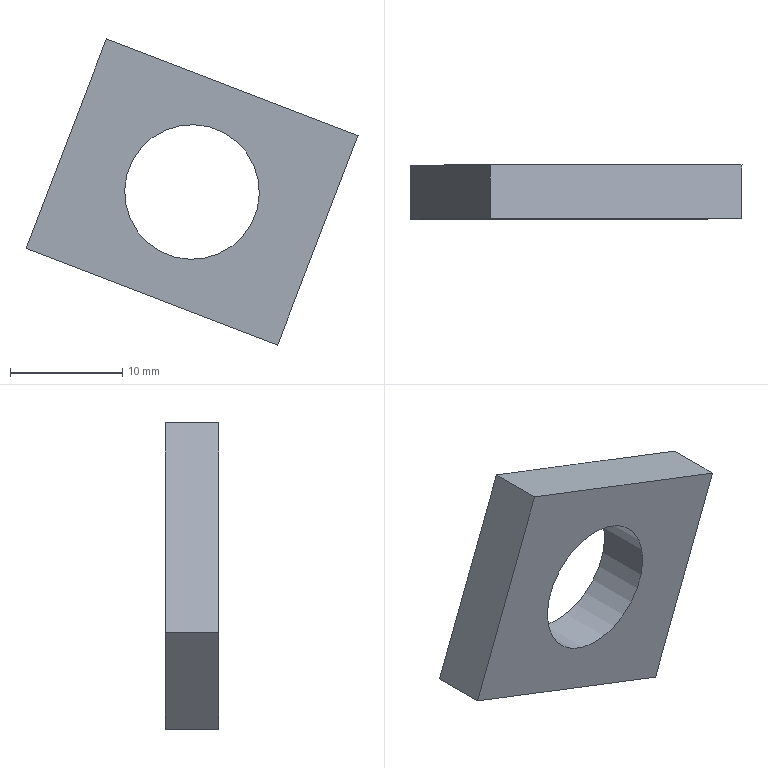Part | STEP file | P011002L001-005 | 1 solid | 7 faces | box 29.573 x 4.8 x 27.272 mm | volume 1761 mm3 | plane 6 | cylinder 1 | commonest cylinder face diameters 12 x1
STEP:
#1=CARTESIAN_POINT('',(0.,0.,0.));
#2=DIRECTION('',(0.,0.,1.));
#3=DIRECTION('',(1.,0.,0.));
#4=AXIS2_PLACEMENT_3D('',#1,#2,#3);
#5=CARTESIAN_POINT('',(-86.963,86.76,-310.6));
#6=VERTEX_POINT('',#5);
#7=CARTESIAN_POINT('',(-64.557,86.76,-319.201));
#8=VERTEX_POINT('',#7);
#9=CARTESIAN_POINT('',(-86.963,86.76,-310.6));
#10=DIRECTION('',(0.9336,0.000000025,-0.3584));
#11=VECTOR('',#10,1.);
#12=LINE('',#9,#11);
#13=CARTESIAN_POINT('',(-77.518,86.76,-285.304));
#14=DIRECTION('',(0.00000001,1.,0.000000094));
#15=DIRECTION('',(0.2588,-0.000000093,0.9659));
#16=AXIS2_PLACEMENT_3D('',#13,#14,#15);
#17=PLANE('',#16);
#18=CARTESIAN_POINT('',(-26.878,-2.576));
#19=DIRECTION('',(-0.1045,0.9945));
#20=VECTOR('',#19,1.);
#21=LINE('',#18,#20);
#22=(GEOMETRIC_REPRESENTATION_CONTEXT(2)PARAMETRIC_REPRESENTATION_CONTEXT()REPRESENTATION_CONTEXT('',''));
#23=DEFINITIONAL_REPRESENTATION('',(#21),#22);
#24=PCURVE('',#17,#23);
#25=CARTESIAN_POINT('',(-86.963,112.76,-310.6));
#26=DIRECTION('',(-0.3584,0.000000186,-0.9336));
#27=DIRECTION('',(-0.9336,-0.000000025,0.3584));
#28=AXIS2_PLACEMENT_3D('',#25,#26,#27);
#29=PLANE('',#28);
#30=CARTESIAN_POINT('',(0.,-26.));
#31=DIRECTION('',(-1.,0.));
#32=VECTOR('',#31,1.);
#33=LINE('',#30,#32);
#34=(GEOMETRIC_REPRESENTATION_CONTEXT(2)PARAMETRIC_REPRESENTATION_CONTEXT()REPRESENTATION_CONTEXT('',''));
#35=DEFINITIONAL_REPRESENTATION('',(#33),#34);
#36=PCURVE('',#29,#35);
#37=SURFACE_CURVE('',#12,(#24,#36),.PCURVE_S1.);
#38=EDGE_CURVE('',#6,#8,#37,.T.);
#39=ORIENTED_EDGE('',*,*,#38,.F.);
#40=CARTESIAN_POINT('',(-79.795,86.76,-291.928));
#41=VERTEX_POINT('',#40);
#42=CARTESIAN_POINT('',(-79.795,86.76,-291.928));
#43=DIRECTION('',(-0.3584,0.000000091,-0.9336));
#44=VECTOR('',#43,1.);
#45=LINE('',#42,#44);
#46=CARTESIAN_POINT('',(-6.988,-0.4856));
#47=DIRECTION('',(-0.9945,-0.1045));
#48=VECTOR('',#47,1.);
#49=LINE('',#46,#48);
#50=(GEOMETRIC_REPRESENTATION_CONTEXT(2)PARAMETRIC_REPRESENTATION_CONTEXT()REPRESENTATION_CONTEXT('',''));
#51=DEFINITIONAL_REPRESENTATION('',(#49),#50);
#52=PCURVE('',#17,#51);
#53=CARTESIAN_POINT('',(-79.795,112.76,-291.928));
#54=DIRECTION('',(-0.9336,-0.000000025,0.3584));
#55=DIRECTION('',(0.3584,-0.000000186,0.9336));
#56=AXIS2_PLACEMENT_3D('',#53,#54,#55);
#57=PLANE('',#56);
#58=CARTESIAN_POINT('',(0.000002462,-26.));
#59=DIRECTION('',(-1.,-0.000000095));
#60=VECTOR('',#59,1.);
#61=LINE('',#58,#60);
#62=(GEOMETRIC_REPRESENTATION_CONTEXT(2)PARAMETRIC_REPRESENTATION_CONTEXT()REPRESENTATION_CONTEXT('',''));
#63=DEFINITIONAL_REPRESENTATION('',(#61),#62);
#64=PCURVE('',#57,#63);
#65=SURFACE_CURVE('',#45,(#52,#64),.PCURVE_S1.);
#66=EDGE_CURVE('',#41,#6,#65,.T.);
#67=ORIENTED_EDGE('',*,*,#66,.F.);
#68=CARTESIAN_POINT('',(-57.389,86.76,-300.529));
#69=VERTEX_POINT('',#68);
#70=CARTESIAN_POINT('',(-80.026,86.76,-291.839));
#71=DIRECTION('',(0.9336,0.000000025,-0.3584));
#72=VECTOR('',#71,1.);
#73=LINE('',#70,#72);
#74=CARTESIAN_POINT('',(-6.962,-0.7317));
#75=DIRECTION('',(-0.1045,0.9945));
#76=VECTOR('',#75,1.);
#77=LINE('',#74,#76);
#78=(GEOMETRIC_REPRESENTATION_CONTEXT(2)PARAMETRIC_REPRESENTATION_CONTEXT()REPRESENTATION_CONTEXT('',''));
#79=DEFINITIONAL_REPRESENTATION('',(#77),#78);
#80=PCURVE('',#17,#79);
#81=CARTESIAN_POINT('',(-57.389,112.76,-300.529));
#82=DIRECTION('',(0.3584,-0.000000186,0.9336));
#83=DIRECTION('',(0.9336,0.000000025,-0.3584));
#84=AXIS2_PLACEMENT_3D('',#81,#82,#83);
#85=PLANE('',#84);
#86=CARTESIAN_POINT('',(-24.247,-26.));
#87=DIRECTION('',(1.,0.));
#88=VECTOR('',#87,1.);
#89=LINE('',#86,#88);
#90=(GEOMETRIC_REPRESENTATION_CONTEXT(2)PARAMETRIC_REPRESENTATION_CONTEXT()REPRESENTATION_CONTEXT('',''));
#91=DEFINITIONAL_REPRESENTATION('',(#89),#90);
#92=PCURVE('',#85,#91);
#93=SURFACE_CURVE('',#73,(#80,#92),.PCURVE_S1.);
#94=EDGE_CURVE('',#41,#69,#93,.T.);
#95=ORIENTED_EDGE('',*,*,#94,.T.);
#96=CARTESIAN_POINT('',(-54.881,86.76,-293.994));
#97=DIRECTION('',(-0.3584,0.000000091,-0.9336));
#98=VECTOR('',#97,1.);
#99=LINE('',#96,#98);
#100=CARTESIAN_POINT('',(-2.535,24.115));
#101=DIRECTION('',(-0.9945,-0.1045));
#102=VECTOR('',#101,1.);
#103=LINE('',#100,#102);
#104=(GEOMETRIC_REPRESENTATION_CONTEXT(2)PARAMETRIC_REPRESENTATION_CONTEXT()REPRESENTATION_CONTEXT('',''));
#105=DEFINITIONAL_REPRESENTATION('',(#103),#104);
#106=PCURVE('',#17,#105);
#107=CARTESIAN_POINT('',(-64.557,112.76,-319.201));
#108=DIRECTION('',(0.9336,0.000000025,-0.3584));
#109=DIRECTION('',(-0.3584,0.000000186,-0.9336));
#110=AXIS2_PLACEMENT_3D('',#107,#108,#109);
#111=PLANE('',#110);
#112=CARTESIAN_POINT('',(-27.,-26.));
#113=DIRECTION('',(1.,-0.000000095));
#114=VECTOR('',#113,1.);
#115=LINE('',#112,#114);
#116=(GEOMETRIC_REPRESENTATION_CONTEXT(2)PARAMETRIC_REPRESENTATION_CONTEXT()REPRESENTATION_CONTEXT('',''));
#117=DEFINITIONAL_REPRESENTATION('',(#115),#116);
#118=PCURVE('',#111,#117);
#119=SURFACE_CURVE('',#99,(#106,#118),.PCURVE_S1.);
#120=EDGE_CURVE('',#69,#8,#119,.T.);
#121=ORIENTED_EDGE('',*,*,#120,.T.);
#122=EDGE_LOOP('',(#39,#67,#95,#121));
#123=FACE_BOUND('',#122,.T.);
#124=CARTESIAN_POINT('',(-70.623,86.76,-299.769));
#125=VERTEX_POINT('',#124);
#126=CARTESIAN_POINT('',(-72.176,86.76,-305.564));
#127=DIRECTION('',(-0.00000001,-1.,-0.000000094));
#128=DIRECTION('',(0.2588,-0.000000093,0.9659));
#129=AXIS2_PLACEMENT_3D('',#126,#127,#128);
#130=CIRCLE('',#129,6.);
#131=CARTESIAN_POINT('',(-12.187,10.403));
#132=CARTESIAN_POINT('',(-12.187,0.01107));
#133=CARTESIAN_POINT('',(-21.187,5.207));
#134=CARTESIAN_POINT('',(-30.187,10.403));
#135=CARTESIAN_POINT('',(-21.187,15.6));
#136=CARTESIAN_POINT('',(-12.187,20.796));
#137=CARTESIAN_POINT('',(-12.187,10.403));
#138=(BOUNDED_CURVE()B_SPLINE_CURVE(2,(#131,#132,#133,#134,#135,#136,#137),.UNSPECIFIED.,.T.,.F.)B_SPLINE_CURVE_WITH_KNOTS((1,2,2,2,2,1),(-2.094,0.,2.094,4.189,6.283,8.378),.UNSPECIFIED.)CURVE()GEOMETRIC_REPRESENTATION_ITEM()RATIONAL_B_SPLINE_CURVE((1.,0.5,1.,0.5,1.,0.5,1.))REPRESENTATION_ITEM(''));
#139=(GEOMETRIC_REPRESENTATION_CONTEXT(2)PARAMETRIC_REPRESENTATION_CONTEXT()REPRESENTATION_CONTEXT('',''));
#140=DEFINITIONAL_REPRESENTATION('',(#138),#139);
#141=PCURVE('',#17,#140);
#142=CARTESIAN_POINT('',(-72.176,56.46,-305.564));
#143=DIRECTION('',(0.00000001,1.,0.000000094));
#144=DIRECTION('',(0.2588,-0.000000093,0.9659));
#145=AXIS2_PLACEMENT_3D('',#142,#143,#144);
#146=CYLINDRICAL_SURFACE('',#145,6.);
#147=CARTESIAN_POINT('',(6.283,30.3));
#148=DIRECTION('',(-1.,0.));
#149=VECTOR('',#148,1.);
#150=LINE('',#147,#149);
#151=(GEOMETRIC_REPRESENTATION_CONTEXT(2)PARAMETRIC_REPRESENTATION_CONTEXT()REPRESENTATION_CONTEXT('',''));
#152=DEFINITIONAL_REPRESENTATION('',(#150),#151);
#153=PCURVE('',#146,#152);
#154=SURFACE_CURVE('',#130,(#141,#153),.PCURVE_S1.);
#155=EDGE_CURVE('',#125,#125,#154,.T.);
#156=ORIENTED_EDGE('',*,*,#155,.T.);
#157=EDGE_LOOP('',(#156));
#158=FACE_BOUND('',#157,.T.);
#159=ADVANCED_FACE('',(#123,#158),#17,.T.);
#160=CARTESIAN_POINT('',(-70.623,81.96,-299.769));
#161=VERTEX_POINT('',#160);
#162=CARTESIAN_POINT('',(-72.176,81.96,-305.564));
#163=DIRECTION('',(-0.00000001,-1.,-0.000000094));
#164=DIRECTION('',(0.2588,-0.000000093,0.9659));
#165=AXIS2_PLACEMENT_3D('',#162,#163,#164);
#166=CIRCLE('',#165,6.);
#167=CARTESIAN_POINT('',(-77.518,81.96,-285.304));
#168=DIRECTION('',(0.00000001,1.,0.000000094));
#169=DIRECTION('',(0.2588,-0.000000093,0.9659));
#170=AXIS2_PLACEMENT_3D('',#167,#168,#169);
#171=PLANE('',#170);
#172=CARTESIAN_POINT('',(-12.187,10.403));
#173=CARTESIAN_POINT('',(-12.187,0.01107));
#174=CARTESIAN_POINT('',(-21.187,5.207));
#175=CARTESIAN_POINT('',(-30.187,10.403));
#176=CARTESIAN_POINT('',(-21.187,15.6));
#177=CARTESIAN_POINT('',(-12.187,20.796));
#178=CARTESIAN_POINT('',(-12.187,10.403));
#179=(BOUNDED_CURVE()B_SPLINE_CURVE(2,(#172,#173,#174,#175,#176,#177,#178),.UNSPECIFIED.,.T.,.F.)B_SPLINE_CURVE_WITH_KNOTS((1,2,2,2,2,1),(-2.094,0.,2.094,4.189,6.283,8.378),.UNSPECIFIED.)CURVE()GEOMETRIC_REPRESENTATION_ITEM()RATIONAL_B_SPLINE_CURVE((1.,0.5,1.,0.5,1.,0.5,1.))REPRESENTATION_ITEM(''));
#180=(GEOMETRIC_REPRESENTATION_CONTEXT(2)PARAMETRIC_REPRESENTATION_CONTEXT()REPRESENTATION_CONTEXT('',''));
#181=DEFINITIONAL_REPRESENTATION('',(#179),#180);
#182=PCURVE('',#171,#181);
#183=CARTESIAN_POINT('',(6.283,25.5));
#184=DIRECTION('',(-1.,0.));
#185=VECTOR('',#184,1.);
#186=LINE('',#183,#185);
#187=(GEOMETRIC_REPRESENTATION_CONTEXT(2)PARAMETRIC_REPRESENTATION_CONTEXT()REPRESENTATION_CONTEXT('',''));
#188=DEFINITIONAL_REPRESENTATION('',(#186),#187);
#189=PCURVE('',#146,#188);
#190=SURFACE_CURVE('',#166,(#182,#189),.PCURVE_S1.);
#191=EDGE_CURVE('',#161,#161,#190,.T.);
#192=ORIENTED_EDGE('',*,*,#191,.F.);
#193=EDGE_LOOP('',(#192));
#194=FACE_BOUND('',#193,.T.);
#195=CARTESIAN_POINT('',(-86.963,81.96,-310.6));
#196=VERTEX_POINT('',#195);
#197=CARTESIAN_POINT('',(-64.557,81.96,-319.201));
#198=VERTEX_POINT('',#197);
#199=CARTESIAN_POINT('',(-86.963,81.96,-310.6));
#200=DIRECTION('',(0.9336,0.000000025,-0.3584));
#201=VECTOR('',#200,1.);
#202=LINE('',#199,#201);
#203=CARTESIAN_POINT('',(-26.878,-2.576));
#204=DIRECTION('',(-0.1045,0.9945));
#205=VECTOR('',#204,1.);
#206=LINE('',#203,#205);
#207=(GEOMETRIC_REPRESENTATION_CONTEXT(2)PARAMETRIC_REPRESENTATION_CONTEXT()REPRESENTATION_CONTEXT('',''));
#208=DEFINITIONAL_REPRESENTATION('',(#206),#207);
#209=PCURVE('',#171,#208);
#210=CARTESIAN_POINT('',(0.,-30.8));
#211=DIRECTION('',(-1.,0.));
#212=VECTOR('',#211,1.);
#213=LINE('',#210,#212);
#214=(GEOMETRIC_REPRESENTATION_CONTEXT(2)PARAMETRIC_REPRESENTATION_CONTEXT()REPRESENTATION_CONTEXT('',''));
#215=DEFINITIONAL_REPRESENTATION('',(#213),#214);
#216=PCURVE('',#29,#215);
#217=SURFACE_CURVE('',#202,(#209,#216),.PCURVE_S1.);
#218=EDGE_CURVE('',#196,#198,#217,.T.);
#219=ORIENTED_EDGE('',*,*,#218,.T.);
#220=CARTESIAN_POINT('',(-57.389,81.96,-300.529));
#221=VERTEX_POINT('',#220);
#222=CARTESIAN_POINT('',(-54.881,81.96,-293.994));
#223=DIRECTION('',(-0.3584,0.000000091,-0.9336));
#224=VECTOR('',#223,1.);
#225=LINE('',#222,#224);
#226=CARTESIAN_POINT('',(-2.535,24.115));
#227=DIRECTION('',(-0.9945,-0.1045));
#228=VECTOR('',#227,1.);
#229=LINE('',#226,#228);
#230=(GEOMETRIC_REPRESENTATION_CONTEXT(2)PARAMETRIC_REPRESENTATION_CONTEXT()REPRESENTATION_CONTEXT('',''));
#231=DEFINITIONAL_REPRESENTATION('',(#229),#230);
#232=PCURVE('',#171,#231);
#233=CARTESIAN_POINT('',(-27.,-30.8));
#234=DIRECTION('',(1.,-0.000000095));
#235=VECTOR('',#234,1.);
#236=LINE('',#233,#235);
#237=(GEOMETRIC_REPRESENTATION_CONTEXT(2)PARAMETRIC_REPRESENTATION_CONTEXT()REPRESENTATION_CONTEXT('',''));
#238=DEFINITIONAL_REPRESENTATION('',(#236),#237);
#239=PCURVE('',#111,#238);
#240=SURFACE_CURVE('',#225,(#232,#239),.PCURVE_S1.);
#241=EDGE_CURVE('',#221,#198,#240,.T.);
#242=ORIENTED_EDGE('',*,*,#241,.F.);
#243=CARTESIAN_POINT('',(-79.795,81.96,-291.928));
#244=VERTEX_POINT('',#243);
#245=CARTESIAN_POINT('',(-80.026,81.96,-291.839));
#246=DIRECTION('',(0.9336,0.000000025,-0.3584));
#247=VECTOR('',#246,1.);
#248=LINE('',#245,#247);
#249=CARTESIAN_POINT('',(-6.962,-0.7317));
#250=DIRECTION('',(-0.1045,0.9945));
#251=VECTOR('',#250,1.);
#252=LINE('',#249,#251);
#253=(GEOMETRIC_REPRESENTATION_CONTEXT(2)PARAMETRIC_REPRESENTATION_CONTEXT()REPRESENTATION_CONTEXT('',''));
#254=DEFINITIONAL_REPRESENTATION('',(#252),#253);
#255=PCURVE('',#171,#254);
#256=CARTESIAN_POINT('',(-24.247,-30.8));
#257=DIRECTION('',(1.,0.));
#258=VECTOR('',#257,1.);
#259=LINE('',#256,#258);
#260=(GEOMETRIC_REPRESENTATION_CONTEXT(2)PARAMETRIC_REPRESENTATION_CONTEXT()REPRESENTATION_CONTEXT('',''));
#261=DEFINITIONAL_REPRESENTATION('',(#259),#260);
#262=PCURVE('',#85,#261);
#263=SURFACE_CURVE('',#248,(#255,#262),.PCURVE_S1.);
#264=EDGE_CURVE('',#244,#221,#263,.T.);
#265=ORIENTED_EDGE('',*,*,#264,.F.);
#266=CARTESIAN_POINT('',(-79.795,81.96,-291.928));
#267=DIRECTION('',(-0.3584,0.000000091,-0.9336));
#268=VECTOR('',#267,1.);
#269=LINE('',#266,#268);
#270=CARTESIAN_POINT('',(-6.988,-0.4856));
#271=DIRECTION('',(-0.9945,-0.1045));
#272=VECTOR('',#271,1.);
#273=LINE('',#270,#272);
#274=(GEOMETRIC_REPRESENTATION_CONTEXT(2)PARAMETRIC_REPRESENTATION_CONTEXT()REPRESENTATION_CONTEXT('',''));
#275=DEFINITIONAL_REPRESENTATION('',(#273),#274);
#276=PCURVE('',#171,#275);
#277=CARTESIAN_POINT('',(0.000002916,-30.8));
#278=DIRECTION('',(-1.,-0.000000095));
#279=VECTOR('',#278,1.);
#280=LINE('',#277,#279);
#281=(GEOMETRIC_REPRESENTATION_CONTEXT(2)PARAMETRIC_REPRESENTATION_CONTEXT()REPRESENTATION_CONTEXT('',''));
#282=DEFINITIONAL_REPRESENTATION('',(#280),#281);
#283=PCURVE('',#57,#282);
#284=SURFACE_CURVE('',#269,(#276,#283),.PCURVE_S1.);
#285=EDGE_CURVE('',#244,#196,#284,.T.);
#286=ORIENTED_EDGE('',*,*,#285,.T.);
#287=EDGE_LOOP('',(#219,#242,#265,#286));
#288=FACE_BOUND('',#287,.T.);
#289=ADVANCED_FACE('',(#194,#288),#171,.F.);
#290=CARTESIAN_POINT('',(-79.795,112.76,-291.928));
#291=DIRECTION('',(0.000000044,1.,0.000000183));
#292=VECTOR('',#291,1.);
#293=LINE('',#290,#292);
#294=CARTESIAN_POINT('',(-24.,0.));
#295=DIRECTION('',(0.,1.));
#296=VECTOR('',#295,1.);
#297=LINE('',#294,#296);
#298=(GEOMETRIC_REPRESENTATION_CONTEXT(2)PARAMETRIC_REPRESENTATION_CONTEXT()REPRESENTATION_CONTEXT('',''));
#299=DEFINITIONAL_REPRESENTATION('',(#297),#298);
#300=PCURVE('',#85,#299);
#301=CARTESIAN_POINT('',(0.,0.));
#302=DIRECTION('',(0.,1.));
#303=VECTOR('',#302,1.);
#304=LINE('',#301,#303);
#305=(GEOMETRIC_REPRESENTATION_CONTEXT(2)PARAMETRIC_REPRESENTATION_CONTEXT()REPRESENTATION_CONTEXT('',''));
#306=DEFINITIONAL_REPRESENTATION('',(#304),#305);
#307=PCURVE('',#57,#306);
#308=SURFACE_CURVE('',#293,(#300,#307),.PCURVE_S1.);
#309=EDGE_CURVE('',#244,#41,#308,.T.);
#310=ORIENTED_EDGE('',*,*,#309,.F.);
#311=ORIENTED_EDGE('',*,*,#264,.T.);
#312=CARTESIAN_POINT('',(-57.389,112.76,-300.529));
#313=DIRECTION('',(0.000000044,1.,0.000000183));
#314=VECTOR('',#313,1.);
#315=LINE('',#312,#314);
#316=CARTESIAN_POINT('',(0.,0.));
#317=DIRECTION('',(0.,1.));
#318=VECTOR('',#317,1.);
#319=LINE('',#316,#318);
#320=(GEOMETRIC_REPRESENTATION_CONTEXT(2)PARAMETRIC_REPRESENTATION_CONTEXT()REPRESENTATION_CONTEXT('',''));
#321=DEFINITIONAL_REPRESENTATION('',(#319),#320);
#322=PCURVE('',#85,#321);
#323=CARTESIAN_POINT('',(-20.,0.));
#324=DIRECTION('',(0.,1.));
#325=VECTOR('',#324,1.);
#326=LINE('',#323,#325);
#327=(GEOMETRIC_REPRESENTATION_CONTEXT(2)PARAMETRIC_REPRESENTATION_CONTEXT()REPRESENTATION_CONTEXT('',''));
#328=DEFINITIONAL_REPRESENTATION('',(#326),#327);
#329=PCURVE('',#111,#328);
#330=SURFACE_CURVE('',#315,(#322,#329),.PCURVE_S1.);
#331=EDGE_CURVE('',#221,#69,#330,.T.);
#332=ORIENTED_EDGE('',*,*,#331,.T.);
#333=ORIENTED_EDGE('',*,*,#94,.F.);
#334=EDGE_LOOP('',(#310,#311,#332,#333));
#335=FACE_BOUND('',#334,.T.);
#336=ADVANCED_FACE('',(#335),#85,.T.);
#337=ORIENTED_EDGE('',*,*,#331,.F.);
#338=ORIENTED_EDGE('',*,*,#241,.T.);
#339=CARTESIAN_POINT('',(-64.557,112.76,-319.201));
#340=DIRECTION('',(0.000000044,1.,0.000000183));
#341=VECTOR('',#340,1.);
#342=LINE('',#339,#341);
#343=CARTESIAN_POINT('',(0.,0.));
#344=DIRECTION('',(0.,1.));
#345=VECTOR('',#344,1.);
#346=LINE('',#343,#345);
#347=(GEOMETRIC_REPRESENTATION_CONTEXT(2)PARAMETRIC_REPRESENTATION_CONTEXT()REPRESENTATION_CONTEXT('',''));
#348=DEFINITIONAL_REPRESENTATION('',(#346),#347);
#349=PCURVE('',#111,#348);
#350=CARTESIAN_POINT('',(-24.,0.));
#351=DIRECTION('',(0.,1.));
#352=VECTOR('',#351,1.);
#353=LINE('',#350,#352);
#354=(GEOMETRIC_REPRESENTATION_CONTEXT(2)PARAMETRIC_REPRESENTATION_CONTEXT()REPRESENTATION_CONTEXT('',''));
#355=DEFINITIONAL_REPRESENTATION('',(#353),#354);
#356=PCURVE('',#29,#355);
#357=SURFACE_CURVE('',#342,(#349,#356),.PCURVE_S1.);
#358=EDGE_CURVE('',#198,#8,#357,.T.);
#359=ORIENTED_EDGE('',*,*,#358,.T.);
#360=ORIENTED_EDGE('',*,*,#120,.F.);
#361=EDGE_LOOP('',(#337,#338,#359,#360));
#362=FACE_BOUND('',#361,.T.);
#363=ADVANCED_FACE('',(#362),#111,.T.);
#364=ORIENTED_EDGE('',*,*,#358,.F.);
#365=ORIENTED_EDGE('',*,*,#218,.F.);
#366=CARTESIAN_POINT('',(-86.963,112.76,-310.6));
#367=DIRECTION('',(0.000000044,1.,0.000000183));
#368=VECTOR('',#367,1.);
#369=LINE('',#366,#368);
#370=CARTESIAN_POINT('',(0.,0.));
#371=DIRECTION('',(0.,1.));
#372=VECTOR('',#371,1.);
#373=LINE('',#370,#372);
#374=(GEOMETRIC_REPRESENTATION_CONTEXT(2)PARAMETRIC_REPRESENTATION_CONTEXT()REPRESENTATION_CONTEXT('',''));
#375=DEFINITIONAL_REPRESENTATION('',(#373),#374);
#376=PCURVE('',#29,#375);
#377=CARTESIAN_POINT('',(-20.,0.));
#378=DIRECTION('',(0.,1.));
#379=VECTOR('',#378,1.);
#380=LINE('',#377,#379);
#381=(GEOMETRIC_REPRESENTATION_CONTEXT(2)PARAMETRIC_REPRESENTATION_CONTEXT()REPRESENTATION_CONTEXT('',''));
#382=DEFINITIONAL_REPRESENTATION('',(#380),#381);
#383=PCURVE('',#57,#382);
#384=SURFACE_CURVE('',#369,(#376,#383),.PCURVE_S1.);
#385=EDGE_CURVE('',#196,#6,#384,.T.);
#386=ORIENTED_EDGE('',*,*,#385,.T.);
#387=ORIENTED_EDGE('',*,*,#38,.T.);
#388=EDGE_LOOP('',(#364,#365,#386,#387));
#389=FACE_BOUND('',#388,.T.);
#390=ADVANCED_FACE('',(#389),#29,.T.);
#391=ORIENTED_EDGE('',*,*,#285,.F.);
#392=ORIENTED_EDGE('',*,*,#309,.T.);
#393=ORIENTED_EDGE('',*,*,#66,.T.);
#394=ORIENTED_EDGE('',*,*,#385,.F.);
#395=EDGE_LOOP('',(#391,#392,#393,#394));
#396=FACE_BOUND('',#395,.T.);
#397=ADVANCED_FACE('',(#396),#57,.T.);
#398=ORIENTED_EDGE('',*,*,#191,.F.);
#399=CARTESIAN_POINT('',(-70.623,81.96,-299.769));
#400=CARTESIAN_POINT('',(-70.623,86.76,-299.769));
#401=B_SPLINE_CURVE_WITH_KNOTS('',1,(#399,#400),.UNSPECIFIED.,.F.,.F.,(2,2),(25.5,30.3),.PIECEWISE_BEZIER_KNOTS.);
#402=CARTESIAN_POINT('',(6.283,0.));
#403=DIRECTION('',(0.,1.));
#404=VECTOR('',#403,1.);
#405=LINE('',#402,#404);
#406=(GEOMETRIC_REPRESENTATION_CONTEXT(2)PARAMETRIC_REPRESENTATION_CONTEXT()REPRESENTATION_CONTEXT('',''));
#407=DEFINITIONAL_REPRESENTATION('',(#405),#406);
#408=PCURVE('',#146,#407);
#409=CARTESIAN_POINT('',(0.,0.));
#410=DIRECTION('',(0.,1.));
#411=VECTOR('',#410,1.);
#412=LINE('',#409,#411);
#413=(GEOMETRIC_REPRESENTATION_CONTEXT(2)PARAMETRIC_REPRESENTATION_CONTEXT()REPRESENTATION_CONTEXT('',''));
#414=DEFINITIONAL_REPRESENTATION('',(#412),#413);
#415=PCURVE('',#146,#414);
#416=SEAM_CURVE('',#401,(#408,#415),.PCURVE_S1.);
#417=EDGE_CURVE('',#161,#125,#416,.T.);
#418=ORIENTED_EDGE('',*,*,#417,.T.);
#419=ORIENTED_EDGE('',*,*,#155,.T.);
#420=ORIENTED_EDGE('',*,*,#417,.F.);
#421=EDGE_LOOP('',(#398,#418,#419,#420));
#422=FACE_BOUND('',#421,.F.);
#423=ADVANCED_FACE('',(#422),#146,.F.);
#424=CLOSED_SHELL('',(#159,#289,#336,#363,#390,#397,#423));
#425=MANIFOLD_SOLID_BREP('',#424);
#426=(LENGTH_UNIT()NAMED_UNIT(*)SI_UNIT(.MILLI.,.METRE.));
#427=UNCERTAINTY_MEASURE_WITH_UNIT(LENGTH_MEASURE(0.000002),#426,'','');
#428=(NAMED_UNIT(*)PLANE_ANGLE_UNIT()SI_UNIT($,.RADIAN.));
#429=(NAMED_UNIT(*)SI_UNIT($,.STERADIAN.)SOLID_ANGLE_UNIT());
#430=(GEOMETRIC_REPRESENTATION_CONTEXT(3)GLOBAL_UNCERTAINTY_ASSIGNED_CONTEXT((#427))GLOBAL_UNIT_ASSIGNED_CONTEXT((#426,#428,#429))REPRESENTATION_CONTEXT('',''));
#431=ADVANCED_BREP_SHAPE_REPRESENTATION('',(#4,#425),#430);